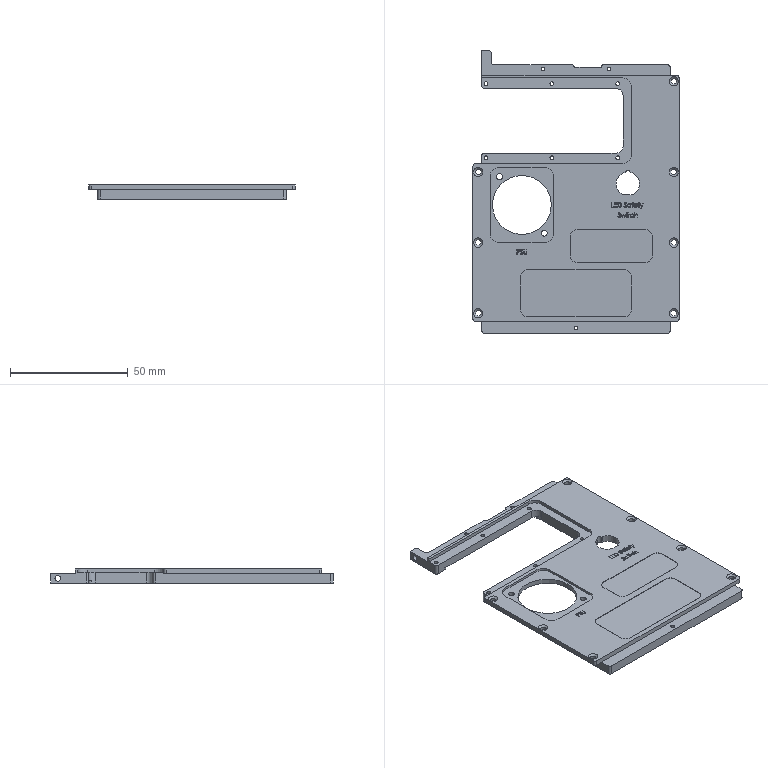NC program | NX | posted with a generic post | part box 87.5 x 120 x 6.001 mm
Lines 5364 to 6313 of 10039:
(ZLEVEL_PROFILE_STEEP , TOOL : D2-6-D4-50-3T-ROUGH)
N10684 T03 M6
N10686 G53
N10688 G17 G0 G90 X-21.7 Y-34.001 B0. C0. S6500 M3
N10690 G43 Z3. H3
N10692 Z-0.326
N10694 G94 G3 X-22.7 Y-35.001 R1. F1500.
N10696 G1 Y-36.95
N10698 X-20.751
N10700 G3 X-19.751 Y-35.95 R1.
N10702 G0 X-21.7 Y-34.001 Z-0.613
N10704 G3 X-22.7 Y-35.001 R1.
N10706 G1 Y-36.95
N10708 X-20.751
N10710 G3 X-19.751 Y-35.95 R1.
N10712 G0 X-21.7 Y-34.001 Z-0.9
N10714 G3 X-22.7 Y-35.001 R1.
N10716 G1 Y-36.95
N10718 X-20.751
N10720 G3 X-19.751 Y-35.95 R1.
N10722 G0 X-21.7 Y-34.001 Z-1.163
N10724 G3 X-22.7 Y-35.001 R1.
N10726 G1 Y-36.95
N10728 X-20.751
N10730 G3 X-19.751 Y-35.95 R1.
N10732 G0 X-21.7 Y-34.001 Z-1.489
N10734 G3 X-22.7 Y-35.001 R1.
N10736 G1 Y-36.95
N10738 X-20.751
N10740 G3 X-19.751 Y-35.95 R1.
N10742 G0 X-21.7 Y-34.001 Z-1.816
N10744 G3 X-22.7 Y-35.001 R1.
N10746 G1 Y-36.95
N10748 X-20.751
N10750 G3 X-19.751 Y-35.95 R1.
N10752 G0 X-21.7 Y-34.001 Z-2.087
N10754 G3 X-22.7 Y-35.001 R1.
N10756 G1 Y-36.95
N10758 X-20.751
N10760 G3 X-19.751 Y-35.95 R1.
N10762 G0 X-21.7 Y-34.001 Z-2.358
N10764 G3 X-22.7 Y-35.001 R1.
N10766 G1 Y-36.95
N10768 X-20.751
N10770 G3 X-19.751 Y-35.95 R1.
N10772 G0 X-21.7 Y-34.001 Z-2.629
N10774 G3 X-22.7 Y-35.001 R1.
N10776 G1 Y-36.95
N10778 X-20.751
N10780 G3 X-19.751 Y-35.95 R1.
N10782 G0 X-21.7 Y-34.001 Z-2.9
N10784 G3 X-22.7 Y-35.001 R1.
N10786 G1 Y-36.95
N10788 X-20.751
N10790 G3 X-19.751 Y-35.95 R1.
N10792 G0 Z3.1
N10794 X9.125
N10796 Z-0.326
N10798 G3 X10.125 Y-36.95 R1.
N10800 G1 X11.45
N10802 Y-36.75
N10804 G2 X11.574 Y-36.048 R2.05
N10806 G3 X11.126 Y-34.835 R1.
N10808 G0 X9.125 Y-35.95 Z-0.613
N10810 G3 X10.125 Y-36.95 R1.
N10812 G1 X11.45
N10814 Y-36.75
N10816 G2 X11.574 Y-36.048 R2.05
N10818 G3 X11.126 Y-34.835 R1.
N10820 G0 X9.125 Y-35.95 Z-0.9
N10822 G3 X10.125 Y-36.95 R1.
N10824 G1 X11.45
N10826 Y-36.75
N10828 G2 X11.574 Y-36.048 R2.05
N10830 G3 X11.126 Y-34.835 R1.
N10832 G0 X9.125 Y-35.95 Z-1.163
N10834 G3 X10.125 Y-36.95 R1.
N10836 G1 X11.45
N10838 Y-36.75
N10840 G2 X11.574 Y-36.048 R2.05
N10842 G3 X11.126 Y-34.835 R1.
N10844 G0 X9.125 Y-35.95 Z-1.489
N10846 G3 X10.125 Y-36.95 R1.
N10848 G1 X11.45
N10850 Y-36.75
N10852 G2 X11.574 Y-36.048 R2.05
N10854 G3 X11.126 Y-34.835 R1.
N10856 G0 X9.125 Y-35.95 Z-1.816
N10858 G3 X10.125 Y-36.95 R1.
N10860 G1 X11.45
N10862 Y-36.75
N10864 G2 X11.574 Y-36.048 R2.05
N10866 G3 X11.126 Y-34.835 R1.
N10868 G0 X9.125 Y-35.95 Z-2.087
N10870 G3 X10.125 Y-36.95 R1.
N10872 G1 X11.45
N10874 Y-36.75
N10876 G2 X11.574 Y-36.048 R2.05
N10878 G3 X11.126 Y-34.835 R1.
N10880 G0 X9.125 Y-35.95 Z-2.358
N10882 G3 X10.125 Y-36.95 R1.
N10884 G1 X11.45
N10886 Y-36.75
N10888 G2 X11.574 Y-36.048 R2.05
N10890 G3 X11.126 Y-34.835 R1.
N10892 G0 X9.125 Y-35.95 Z-2.629
N10894 G3 X10.125 Y-36.95 R1.
N10896 G1 X11.45
N10898 Y-36.75
N10900 G2 X11.574 Y-36.048 R2.05
N10902 G3 X11.126 Y-34.835 R1.
N10904 G0 X9.125 Y-35.95 Z-2.9
N10906 G3 X10.125 Y-36.95 R1.
N10908 G1 X11.45
N10910 Y-36.75
N10912 G2 X11.574 Y-36.048 R2.05
N10914 G3 X11.126 Y-34.835 R1.
N10916 G0 Z3.1
N10918 X11.435 Y-34.505
N10920 Z-0.326
N10922 G3 X12.675 Y-34.873 R1.
N10924 G2 X13.45 Y-34.701 R2.05
N10926 G1 Y-33.533
N10928 G3 X12.45 Y-32.533 R1.
N10930 G0 X11.435 Y-34.505 Z-0.613
N10932 G3 X12.675 Y-34.873 R1.
N10934 G2 X13.45 Y-34.701 R2.05
N10936 G1 Y-33.533
N10938 G3 X12.45 Y-32.533 R1.
N10940 G0 X11.435 Y-34.505 Z-0.9
N10942 G3 X12.675 Y-34.873 R1.
N10944 G2 X13.45 Y-34.701 R2.05
N10946 G1 Y-33.533
N10948 G3 X12.45 Y-32.533 R1.
N10950 G0 X11.435 Y-34.505 Z-1.163
N10952 G3 X12.675 Y-34.873 R1.
N10954 G2 X13.45 Y-34.701 R2.05
N10956 G1 Y-33.533
N10958 G3 X12.45 Y-32.533 R1.
N10960 G0 X11.435 Y-34.505 Z-1.489
N10962 G3 X12.675 Y-34.873 R1.
N10964 G2 X13.45 Y-34.701 R2.05
N10966 G1 Y-33.533
N10968 G3 X12.45 Y-32.533 R1.
N10970 G0 X11.435 Y-34.505 Z-1.816
N10972 G3 X12.675 Y-34.873 R1.
N10974 G2 X13.45 Y-34.701 R2.05
N10976 G1 Y-33.533
N10978 G3 X12.45 Y-32.533 R1.
N10980 G0 X11.435 Y-34.505 Z-2.087
N10982 G3 X12.675 Y-34.873 R1.
N10984 G2 X13.45 Y-34.701 R2.05
N10986 G1 Y-33.533
N10988 G3 X12.45 Y-32.533 R1.
N10990 G0 X11.435 Y-34.505 Z-2.358
N10992 G3 X12.675 Y-34.873 R1.
N10994 G2 X13.45 Y-34.701 R2.05
N10996 G1 Y-33.533
N10998 G3 X12.45 Y-32.533 R1.
N11000 G0 X11.435 Y-34.505 Z-2.629
N11002 G3 X12.675 Y-34.873 R1.
N11004 G2 X13.45 Y-34.701 R2.05
N11006 G1 Y-33.533
N11008 G3 X12.45 Y-32.533 R1.
N11010 G0 X11.435 Y-34.505 Z-2.9
N11012 G3 X12.675 Y-34.873 R1.
N11014 G2 X13.45 Y-34.701 R2.05
N11016 G1 Y-33.533
N11018 G3 X12.45 Y-32.533 R1.
N11020 G0 Z3.1
N11022 Y-15.967
N11024 Z-0.326
N11026 G3 X13.45 Y-14.967 R1.
N11028 G1 Y-13.799
N11030 G2 X12.675 Y-13.627 R2.05
N11032 G3 X11.435 Y-13.995 R1.
N11034 G0 X12.45 Y-15.967 Z-0.613
N11036 G3 X13.45 Y-14.967 R1.
N11038 G1 Y-13.799
N11040 G2 X12.675 Y-13.627 R2.05
N11042 G3 X11.435 Y-13.995 R1.
N11044 G0 X12.45 Y-15.967 Z-0.9
N11046 G3 X13.45 Y-14.967 R1.
N11048 G1 Y-13.799
N11050 G2 X12.675 Y-13.627 R2.05
N11052 G3 X11.435 Y-13.995 R1.
N11054 G0 X12.45 Y-15.967 Z-1.163
N11056 G3 X13.45 Y-14.967 R1.
N11058 G1 Y-13.799
N11060 G2 X12.675 Y-13.627 R2.05
N11062 G3 X11.435 Y-13.995 R1.
N11064 G0 X12.45 Y-15.967 Z-1.489
N11066 G3 X13.45 Y-14.967 R1.
N11068 G1 Y-13.799
N11070 G2 X12.675 Y-13.627 R2.05
N11072 G3 X11.435 Y-13.995 R1.
N11074 G0 X12.45 Y-15.967 Z-1.816
N11076 G3 X13.45 Y-14.967 R1.
N11078 G1 Y-13.799
N11080 G2 X12.675 Y-13.627 R2.05
N11082 G3 X11.435 Y-13.995 R1.
N11084 G0 X12.45 Y-15.967 Z-2.087
N11086 G3 X13.45 Y-14.967 R1.
N11088 G1 Y-13.799
N11090 G2 X12.675 Y-13.627 R2.05
N11092 G3 X11.435 Y-13.995 R1.
N11094 G0 X12.45 Y-15.967 Z-2.358
N11096 G3 X13.45 Y-14.967 R1.
N11098 G1 Y-13.799
N11100 G2 X12.675 Y-13.627 R2.05
N11102 G3 X11.435 Y-13.995 R1.
N11104 G0 X12.45 Y-15.967 Z-2.629
N11106 G3 X13.45 Y-14.967 R1.
N11108 G1 Y-13.799
N11110 G2 X12.675 Y-13.627 R2.05
N11112 G3 X11.435 Y-13.995 R1.
N11114 G0 X12.45 Y-15.967 Z-2.9
N11116 G3 X13.45 Y-14.967 R1.
N11118 G1 Y-13.799
N11120 G2 X12.675 Y-13.627 R2.05
N11122 G3 X11.435 Y-13.995 R1.
N11124 G0 Z3.1
N11126 X10.46 Y-11.999
N11128 Z-0.326
N11130 G3 X11.45 Y-10.999 R1.
N11132 G1 Y-9.05
N11134 X9.501
N11136 G3 X8.501 Y-10.05 R1.
N11138 G0 X10.46 Y-11.999 Z-0.613
N11140 G3 X11.45 Y-10.999 R1.
N11142 G1 Y-9.05
N11144 X9.501
N11146 G3 X8.501 Y-10.05 R1.
N11148 G0 X10.46 Y-11.999 Z-0.9
N11150 G3 X11.45 Y-10.999 R1.
N11152 G1 Y-9.05
N11154 X9.501
N11156 G3 X8.501 Y-10.05 R1.
N11158 G0 X10.46 Y-11.999 Z-1.163
N11160 G3 X11.45 Y-10.999 R1.
N11162 G1 Y-9.05
N11164 X9.501
N11166 G3 X8.501 Y-10.05 R1.
N11168 G0 X10.46 Y-11.999 Z-1.489
N11170 G3 X11.45 Y-10.999 R1.
N11172 G1 Y-9.05
N11174 X9.501
N11176 G3 X8.501 Y-10.05 R1.
N11178 G0 X10.46 Y-11.999 Z-1.816
N11180 G3 X11.45 Y-10.999 R1.
N11182 G1 Y-9.05
N11184 X9.501
N11186 G3 X8.501 Y-10.05 R1.
N11188 G0 X10.46 Y-11.999 Z-2.087
N11190 G3 X11.45 Y-10.999 R1.
N11192 G1 Y-9.05
N11194 X9.501
N11196 G3 X8.501 Y-10.05 R1.
N11198 G0 X10.46 Y-11.999 Z-2.358
N11200 G3 X11.45 Y-10.999 R1.
N11202 G1 Y-9.05
N11204 X9.501
N11206 G3 X8.501 Y-10.05 R1.
N11208 G0 X10.46 Y-11.999 Z-2.629
N11210 G3 X11.45 Y-10.999 R1.
N11212 G1 Y-9.05
N11214 X9.501
N11216 G3 X8.501 Y-10.05 R1.
N11218 G0 X10.46 Y-11.999 Z-2.9
N11220 G3 X11.45 Y-10.999 R1.
N11222 G1 Y-9.05
N11224 X9.501
N11226 G3 X8.501 Y-10.05 R1.
N11228 G0 Z3.1
N11230 X-19.751
N11232 Z-0.326
N11234 G3 X-20.751 Y-9.05 R1.
N11236 G1 X-22.7
N11238 Y-10.999
N11240 G3 X-21.7 Y-11.999 R1.
N11242 G0 X-19.751 Y-10.05 Z-0.613
N11244 G3 X-20.751 Y-9.05 R1.
N11246 G1 X-22.7
N11248 Y-10.999
N11250 G3 X-21.7 Y-11.999 R1.
N11252 G0 X-19.751 Y-10.05 Z-0.9
N11254 G3 X-20.751 Y-9.05 R1.
N11256 G1 X-22.7
N11258 Y-10.999
N11260 G3 X-21.7 Y-11.999 R1.
N11262 G0 X-19.751 Y-10.05 Z-1.163
N11264 G3 X-20.751 Y-9.05 R1.
N11266 G1 X-22.7
N11268 Y-10.999
N11270 G3 X-21.7 Y-11.999 R1.
N11272 G0 X-19.751 Y-10.05 Z-1.489
N11274 G3 X-20.751 Y-9.05 R1.
N11276 G1 X-22.7
N11278 Y-10.999
N11280 G3 X-21.7 Y-11.999 R1.
N11282 G0 X-19.751 Y-10.05 Z-1.816
N11284 G3 X-20.751 Y-9.05 R1.
N11286 G1 X-22.7
N11288 Y-10.999
N11290 G3 X-21.7 Y-11.999 R1.
N11292 G0 X-19.751 Y-10.05 Z-2.087
N11294 G3 X-20.751 Y-9.05 R1.
N11296 G1 X-22.7
N11298 Y-10.999
N11300 G3 X-21.7 Y-11.999 R1.
N11302 G0 X-19.751 Y-10.05 Z-2.358
N11304 G3 X-20.751 Y-9.05 R1.
N11306 G1 X-22.7
N11308 Y-10.999
N11310 G3 X-21.7 Y-11.999 R1.
N11312 G0 X-19.751 Y-10.05 Z-2.629
N11314 G3 X-20.751 Y-9.05 R1.
N11316 G1 X-22.7
N11318 Y-10.999
N11320 G3 X-21.7 Y-11.999 R1.
N11322 G0 X-19.751 Y-10.05 Z-2.9
N11324 G3 X-20.751 Y-9.05 R1.
N11326 G1 X-22.7
N11328 Y-10.999
N11330 G3 X-21.7 Y-11.999 R1.
N11332 G0 Z3.1
N11334 Y-2.001
N11336 Z-0.326
N11338 G3 X-22.7 Y-3.001 R1.
N11340 G1 Y-4.95
N11342 X-20.751
N11344 G3 X-19.751 Y-3.95 R1.
N11346 G0 X-21.7 Y-2.001 Z-0.613
N11348 G3 X-22.7 Y-3.001 R1.
N11350 G1 Y-4.95
N11352 X-20.751
N11354 G3 X-19.751 Y-3.95 R1.
N11356 G0 X-21.7 Y-2.001 Z-0.9
N11358 G3 X-22.7 Y-3.001 R1.
N11360 G1 Y-4.95
N11362 X-20.751
N11364 G3 X-19.751 Y-3.95 R1.
N11366 G0 X-21.7 Y-2.001 Z-1.163
N11368 G3 X-22.7 Y-3.001 R1.
N11370 G1 Y-4.95
N11372 X-20.751
N11374 G3 X-19.751 Y-3.95 R1.
N11376 G0 X-21.7 Y-2.001 Z-1.489
N11378 G3 X-22.7 Y-3.001 R1.
N11380 G1 Y-4.95
N11382 X-20.751
N11384 G3 X-19.751 Y-3.95 R1.
N11386 G0 X-21.7 Y-2.001 Z-1.816
N11388 G3 X-22.7 Y-3.001 R1.
N11390 G1 Y-4.95
N11392 X-20.751
N11394 G3 X-19.751 Y-3.95 R1.
N11396 G0 X-21.7 Y-2.001 Z-2.087
N11398 G3 X-22.7 Y-3.001 R1.
N11400 G1 Y-4.95
N11402 X-20.751
N11404 G3 X-19.751 Y-3.95 R1.
N11406 G0 X-21.7 Y-2.001 Z-2.358
N11408 G3 X-22.7 Y-3.001 R1.
N11410 G1 Y-4.95
N11412 X-20.751
N11414 G3 X-19.751 Y-3.95 R1.
N11416 G0 X-21.7 Y-2.001 Z-2.629
N11418 G3 X-22.7 Y-3.001 R1.
N11420 G1 Y-4.95
N11422 X-20.751
N11424 G3 X-19.751 Y-3.95 R1.
N11426 G0 X-21.7 Y-2.001 Z-2.9
N11428 G3 X-22.7 Y-3.001 R1.
N11430 G1 Y-4.95
N11432 X-20.751
N11434 G3 X-19.751 Y-3.95 R1.
N11436 G0 Z3.1
N11438 X10.501
N11440 Z-0.326
N11442 G3 X11.501 Y-4.95 R1.
N11444 G1 X13.45
N11446 Y-3.001
N11448 G3 X12.45 Y-2.001 R1.
N11450 G0 X10.501 Y-3.95 Z-0.613
N11452 G3 X11.501 Y-4.95 R1.
N11454 G1 X13.45
N11456 Y-3.001
N11458 G3 X12.45 Y-2.001 R1.
N11460 G0 X10.501 Y-3.95 Z-0.9
N11462 G3 X11.501 Y-4.95 R1.
N11464 G1 X13.45
N11466 Y-3.001
N11468 G3 X12.45 Y-2.001 R1.
N11470 G0 X10.501 Y-3.95 Z-1.163
N11472 G3 X11.501 Y-4.95 R1.
N11474 G1 X13.45
N11476 Y-3.001
N11478 G3 X12.45 Y-2.001 R1.
N11480 G0 X10.501 Y-3.95 Z-1.489
N11482 G3 X11.501 Y-4.95 R1.
N11484 G1 X13.45
N11486 Y-3.001
N11488 G3 X12.45 Y-2.001 R1.
N11490 G0 X10.501 Y-3.95 Z-1.816
N11492 G3 X11.501 Y-4.95 R1.
N11494 G1 X13.45
N11496 Y-3.001
N11498 G3 X12.45 Y-2.001 R1.
N11500 G0 X10.501 Y-3.95 Z-2.087
N11502 G3 X11.501 Y-4.95 R1.
N11504 G1 X13.45
N11506 Y-3.001
N11508 G3 X12.45 Y-2.001 R1.
N11510 G0 X10.501 Y-3.95 Z-2.358
N11512 G3 X11.501 Y-4.95 R1.
N11514 G1 X13.45
N11516 Y-3.001
N11518 G3 X12.45 Y-2.001 R1.
N11520 G0 X10.501 Y-3.95 Z-2.629
N11522 G3 X11.501 Y-4.95 R1.
N11524 G1 X13.45
N11526 Y-3.001
N11528 G3 X12.45 Y-2.001 R1.
N11530 G0 X10.501 Y-3.95 Z-2.9
N11532 G3 X11.501 Y-4.95 R1.
N11534 G1 X13.45
N11536 Y-3.001
N11538 G3 X12.45 Y-2.001 R1.
N11540 G0 Z3.1
N11542 Y2.501
N11544 Z-0.326
N11546 G3 X13.45 Y3.501 R1.
N11548 G1 Y5.45
N11550 X11.501
N11552 G3 X10.501 Y4.45 R1.
N11554 G0 X12.45 Y2.501 Z-0.613
N11556 G3 X13.45 Y3.501 R1.
N11558 G1 Y5.45
N11560 X11.501
N11562 G3 X10.501 Y4.45 R1.
N11564 G0 X12.45 Y2.501 Z-0.9
N11566 G3 X13.45 Y3.501 R1.
N11568 G1 Y5.45
N11570 X11.501
N11572 G3 X10.501 Y4.45 R1.
N11574 G0 X12.45 Y2.501 Z-1.163
N11576 G3 X13.45 Y3.501 R1.
N11578 G1 Y5.45
N11580 X11.501
N11582 G3 X10.501 Y4.45 R1.
N11584 G0 X12.45 Y2.501 Z-1.489
N11586 G3 X13.45 Y3.501 R1.
N11588 G1 Y5.45
N11590 X11.501
N11592 G3 X10.501 Y4.45 R1.
N11594 G0 X12.45 Y2.501 Z-1.816
N11596 G3 X13.45 Y3.501 R1.
N11598 G1 Y5.45
N11600 X11.501
N11602 G3 X10.501 Y4.45 R1.
N11604 G0 X12.45 Y2.501 Z-2.087
N11606 G3 X13.45 Y3.501 R1.
N11608 G1 Y5.45
N11610 X11.501
N11612 G3 X10.501 Y4.45 R1.
N11614 G0 X12.45 Y2.501 Z-2.358
N11616 G3 X13.45 Y3.501 R1.
N11618 G1 Y5.45
N11620 X11.501
N11622 G3 X10.501 Y4.45 R1.
N11624 G0 X12.45 Y2.501 Z-2.629
N11626 G3 X13.45 Y3.501 R1.
N11628 G1 Y5.45
N11630 X11.501
N11632 G3 X10.501 Y4.45 R1.
N11634 G0 X12.45 Y2.501 Z-2.9
N11636 G3 X13.45 Y3.501 R1.
N11638 G1 Y5.45
N11640 X11.501
N11642 G3 X10.501 Y4.45 R1.
N11644 G0 Z3.1
N11646 X-19.751
N11648 Z-0.326
N11650 G3 X-20.751 Y5.45 R1.
N11652 G1 X-22.7
N11654 Y3.501
N11656 G3 X-21.7 Y2.501 R1.
N11658 G0 X-19.751 Y4.45 Z-0.613
N11660 G3 X-20.751 Y5.45 R1.
N11662 G1 X-22.7
N11664 Y3.501
N11666 G3 X-21.7 Y2.501 R1.
N11668 G0 X-19.751 Y4.45 Z-0.9
N11670 G3 X-20.751 Y5.45 R1.
N11672 G1 X-22.7
N11674 Y3.501
N11676 G3 X-21.7 Y2.501 R1.
N11678 G0 X-19.751 Y4.45 Z-1.163
N11680 G3 X-20.751 Y5.45 R1.
N11682 G1 X-22.7
N11684 Y3.501
N11686 G3 X-21.7 Y2.501 R1.
N11688 G0 X-19.751 Y4.45 Z-1.489
N11690 G3 X-20.751 Y5.45 R1.
N11692 G1 X-22.7
N11694 Y3.501
N11696 G3 X-21.7 Y2.501 R1.
N11698 G0 X-19.751 Y4.45 Z-1.816
N11700 G3 X-20.751 Y5.45 R1.
N11702 G1 X-22.7
N11704 Y3.501
N11706 G3 X-21.7 Y2.501 R1.
N11708 G0 X-19.751 Y4.45 Z-2.087
N11710 G3 X-20.751 Y5.45 R1.
N11712 G1 X-22.7
N11714 Y3.501
N11716 G3 X-21.7 Y2.501 R1.
N11718 G0 X-19.751 Y4.45 Z-2.358
N11720 G3 X-20.751 Y5.45 R1.
N11722 G1 X-22.7
N11724 Y3.501
N11726 G3 X-21.7 Y2.501 R1.
N11728 G0 X-19.751 Y4.45 Z-2.629
N11730 G3 X-20.751 Y5.45 R1.
N11732 G1 X-22.7
N11734 Y3.501
N11736 G3 X-21.7 Y2.501 R1.
N11738 G0 X-19.751 Y4.45 Z-2.9
N11740 G3 X-20.751 Y5.45 R1.
N11742 G1 X-22.7
N11744 Y3.501
N11746 G3 X-21.7 Y2.501 R1.
N11748 G0 Z3.1
N11750 Y12.499
N11752 Z-0.326
N11754 G3 X-22.7 Y11.499 R1.
N11756 G1 Y9.55
N11758 X-20.751
N11760 G3 X-19.751 Y10.55 R1.
N11762 G0 X-21.7 Y12.499 Z-0.613
N11764 G3 X-22.7 Y11.499 R1.
N11766 G1 Y9.55
N11768 X-20.751
N11770 G3 X-19.751 Y10.55 R1.
N11772 G0 X-21.7 Y12.499 Z-0.9
N11774 G3 X-22.7 Y11.499 R1.
N11776 G1 Y9.55
N11778 X-20.751
N11780 G3 X-19.751 Y10.55 R1.
N11782 G0 X-21.7 Y12.499 Z-1.163
N11784 G3 X-22.7 Y11.499 R1.
N11786 G1 Y9.55
N11788 X-20.751
N11790 G3 X-19.751 Y10.55 R1.
N11792 G0 X-21.7 Y12.499 Z-1.489
N11794 G3 X-22.7 Y11.499 R1.
N11796 G1 Y9.55
N11798 X-20.751
N11800 G3 X-19.751 Y10.55 R1.
N11802 G0 X-21.7 Y12.499 Z-1.816
N11804 G3 X-22.7 Y11.499 R1.
N11806 G1 Y9.55
N11808 X-20.751
N11810 G3 X-19.751 Y10.55 R1.
N11812 G0 X-21.7 Y12.499 Z-2.087
N11814 G3 X-22.7 Y11.499 R1.
N11816 G1 Y9.55
N11818 X-20.751
N11820 G3 X-19.751 Y10.55 R1.
N11822 G0 X-21.7 Y12.499 Z-2.358
N11824 G3 X-22.7 Y11.499 R1.
N11826 G1 Y9.55
N11828 X-20.751
N11830 G3 X-19.751 Y10.55 R1.
N11832 G0 X-21.7 Y12.499 Z-2.629
N11834 G3 X-22.7 Y11.499 R1.
N11836 G1 Y9.55
N11838 X-20.751
N11840 G3 X-19.751 Y10.55 R1.
N11842 G0 X-21.7 Y12.499 Z-2.9
N11844 G3 X-22.7 Y11.499 R1.
N11846 G1 Y9.55
N11848 X-20.751
N11850 G3 X-19.751 Y10.55 R1.
N11852 G0 Z3.1
N11854 X10.501
N11856 Z-0.326
N11858 G3 X11.501 Y9.55 R1.
N11860 G1 X13.45
N11862 Y11.499
N11864 G3 X12.45 Y12.499 R1.
N11866 G0 X10.501 Y10.55 Z-0.613
N11868 G3 X11.501 Y9.55 R1.
N11870 G1 X13.45
N11872 Y11.499
N11874 G3 X12.45 Y12.499 R1.
N11876 G0 X10.501 Y10.55 Z-0.9
N11878 G3 X11.501 Y9.55 R1.
N11880 G1 X13.45
N11882 Y11.499
N11884 G3 X12.45 Y12.499 R1.
N11886 G0 X10.501 Y10.55 Z-1.163
N11888 G3 X11.501 Y9.55 R1.
N11890 G1 X13.45
N11892 Y11.499
N11894 G3 X12.45 Y12.499 R1.
N11896 G0 X10.501 Y10.55 Z-1.489
N11898 G3 X11.501 Y9.55 R1.
N11900 G1 X13.45
N11902 Y11.499
N11904 G3 X12.45 Y12.499 R1.
N11906 G0 X10.501 Y10.55 Z-1.816
N11908 G3 X11.501 Y9.55 R1.
N11910 G1 X13.45
N11912 Y11.499
N11914 G3 X12.45 Y12.499 R1.
N11916 G0 X10.501 Y10.55 Z-2.087
N11918 G3 X11.501 Y9.55 R1.
N11920 G1 X13.45
N11922 Y11.499
N11924 G3 X12.45 Y12.499 R1.
N11926 G0 X10.501 Y10.55 Z-2.358
N11928 G3 X11.501 Y9.55 R1.
N11930 G1 X13.45
N11932 Y11.499
N11934 G3 X12.45 Y12.499 R1.
N11936 G0 X10.501 Y10.55 Z-2.629
N11938 G3 X11.501 Y9.55 R1.
N11940 G1 X13.45
N11942 Y11.499
N11944 G3 X12.45 Y12.499 R1.
N11946 G0 X10.501 Y10.55 Z-2.9
N11948 G3 X11.501 Y9.55 R1.
N11950 G1 X13.45
N11952 Y11.499
N11954 G3 X12.45 Y12.499 R1.
N11956 G0 Z3.1
N11958 Y12.033
N11960 Z-0.326
N11962 G3 X13.45 Y13.033 R1.
N11964 G1 Y14.201
N11966 G2 X12.675 Y14.373 R2.05
N11968 G3 X11.435 Y14.005 R1.
N11970 G0 X12.45 Y12.033 Z-0.613
N11972 G3 X13.45 Y13.033 R1.
N11974 G1 Y14.201
N11976 G2 X12.675 Y14.373 R2.05
N11978 G3 X11.435 Y14.005 R1.
N11980 G0 X12.45 Y12.033 Z-0.9
N11982 G3 X13.45 Y13.033 R1.
N11984 G1 Y14.201
N11986 G2 X12.675 Y14.373 R2.05
N11988 G3 X11.435 Y14.005 R1.
N11990 G0 X12.45 Y12.033 Z-1.163
N11992 G3 X13.45 Y13.033 R1.
N11994 G1 Y14.201
N11996 G2 X12.675 Y14.373 R2.05
N11998 G3 X11.435 Y14.005 R1.
N12000 G0 X12.45 Y12.033 Z-1.489
N12002 G3 X13.45 Y13.033 R1.
N12004 G1 Y14.201
N12006 G2 X12.675 Y14.373 R2.05
N12008 G3 X11.435 Y14.005 R1.
N12010 G0 X12.45 Y12.033 Z-1.816
N12012 G3 X13.45 Y13.033 R1.
N12014 G1 Y14.201
N12016 G2 X12.675 Y14.373 R2.05
N12018 G3 X11.435 Y14.005 R1.
N12020 G0 X12.45 Y12.033 Z-2.087
N12022 G3 X13.45 Y13.033 R1.
N12024 G1 Y14.201
N12026 G2 X12.675 Y14.373 R2.05
N12028 G3 X11.435 Y14.005 R1.
N12030 G0 X12.45 Y12.033 Z-2.358
N12032 G3 X13.45 Y13.033 R1.
N12034 G1 Y14.201
N12036 G2 X12.675 Y14.373 R2.05
N12038 G3 X11.435 Y14.005 R1.
N12040 G0 X12.45 Y12.033 Z-2.629
N12042 G3 X13.45 Y13.033 R1.
N12044 G1 Y14.201
N12046 G2 X12.675 Y14.373 R2.05
N12048 G3 X11.435 Y14.005 R1.
N12050 G0 X12.45 Y12.033 Z-2.9
N12052 G3 X13.45 Y13.033 R1.
N12054 G1 Y14.201
N12056 G2 X12.675 Y14.373 R2.05
N12058 G3 X11.435 Y14.005 R1.
N12060 G0 Z3.1
N12062 Y21.495
N12064 Z-0.326
N12066 G3 X12.675 Y21.127 R1.
N12068 G2 X13.45 Y21.299 R2.05
N12070 G1 Y22.467
N12072 G3 X12.45 Y23.467 R1.
N12074 G0 X11.435 Y21.495 Z-0.613
N12076 G3 X12.675 Y21.127 R1.
N12078 G2 X13.45 Y21.299 R2.05
N12080 G1 Y22.467
N12082 G3 X12.45 Y23.467 R1.
N12084 G0 X11.435 Y21.495 Z-0.9
N12086 G3 X12.675 Y21.127 R1.
N12088 G2 X13.45 Y21.299 R2.05
N12090 G1 Y22.467
N12092 G3 X12.45 Y23.467 R1.
N12094 G0 X11.435 Y21.495 Z-1.163
N12096 G3 X12.675 Y21.127 R1.
N12098 G2 X13.45 Y21.299 R2.05
N12100 G1 Y22.467
N12102 G3 X12.45 Y23.467 R1.
N12104 G0 X11.435 Y21.495 Z-1.489
N12106 G3 X12.675 Y21.127 R1.
N12108 G2 X13.45 Y21.299 R2.05
N12110 G1 Y22.467
N12112 G3 X12.45 Y23.467 R1.
N12114 G0 X11.435 Y21.495 Z-1.816
N12116 G3 X12.675 Y21.127 R1.
N12118 G2 X13.45 Y21.299 R2.05
N12120 G1 Y22.467
N12122 G3 X12.45 Y23.467 R1.
N12124 G0 X11.435 Y21.495 Z-2.087
N12126 G3 X12.675 Y21.127 R1.
N12128 G2 X13.45 Y21.299 R2.05
N12130 G1 Y22.467
N12132 G3 X12.45 Y23.467 R1.
N12134 G0 X11.435 Y21.495 Z-2.358
N12136 G3 X12.675 Y21.127 R1.
N12138 G2 X13.45 Y21.299 R2.05
N12140 G1 Y22.467
N12142 G3 X12.45 Y23.467 R1.
N12144 G0 X11.435 Y21.495 Z-2.629
N12146 G3 X12.675 Y21.127 R1.
N12148 G2 X13.45 Y21.299 R2.05
N12150 G1 Y22.467
N12152 G3 X12.45 Y23.467 R1.
N12154 G0 X11.435 Y21.495 Z-2.9
N12156 G3 X12.675 Y21.127 R1.
N12158 G2 X13.45 Y21.299 R2.05
N12160 G1 Y22.467
N12162 G3 X12.45 Y23.467 R1.
N12164 G0 Z3.1
N12166 Y34.001
N12168 Z-0.326
N12170 G3 X13.45 Y35.001 R1.
N12172 G1 Y36.95
N12174 X11.501
N12176 G3 X10.501 Y35.95 R1.
N12178 G0 X12.45 Y34.001 Z-0.613
N12180 G3 X13.45 Y35.001 R1.
N12182 G1 Y36.95
N12184 X11.501
N12186 G3 X10.501 Y35.95 R1.
N12188 G0 X12.45 Y34.001 Z-0.9
N12190 G3 X13.45 Y35.001 R1.
N12192 G1 Y36.95
N12194 X11.501
N12196 G3 X10.501 Y35.95 R1.
N12198 G0 X12.45 Y34.001 Z-1.163
N12200 G3 X13.45 Y35.001 R1.
N12202 G1 Y36.95
N12204 X11.501
N12206 G3 X10.501 Y35.95 R1.
N12208 G0 X12.45 Y34.001 Z-1.489
N12210 G3 X13.45 Y35.001 R1.
N12212 G1 Y36.95
N12214 X11.501
N12216 G3 X10.501 Y35.95 R1.
N12218 G0 X12.45 Y34.001 Z-1.816
N12220 G3 X13.45 Y35.001 R1.
N12222 G1 Y36.95
N12224 X11.501
N12226 G3 X10.501 Y35.95 R1.
N12228 G0 X12.45 Y34.001 Z-2.087
N12230 G3 X13.45 Y35.001 R1.
N12232 G1 Y36.95
N12234 X11.501
N12236 G3 X10.501 Y35.95 R1.
N12238 G0 X12.45 Y34.001 Z-2.358
N12240 G3 X13.45 Y35.001 R1.
N12242 G1 Y36.95
N12244 X11.501
N12246 G3 X10.501 Y35.95 R1.
N12248 G0 X12.45 Y34.001 Z-2.629
N12250 G3 X13.45 Y35.001 R1.
N12252 G1 Y36.95
N12254 X11.501
N12256 G3 X10.501 Y35.95 R1.
N12258 G0 X12.45 Y34.001 Z-2.9
N12260 G3 X13.45 Y35.001 R1.
N12262 G1 Y36.95
N12264 X11.501
N12266 G3 X10.501 Y35.95 R1.
N12268 G0 Z3.1
N12270 X-19.751
N12272 Z-0.326
N12274 G3 X-20.751 Y36.95 R1.
N12276 G1 X-22.7
N12278 Y35.001
N12280 G3 X-21.7 Y34.001 R1.
N12282 G0 X-19.751 Y35.95 Z-0.613
N12284 G3 X-20.751 Y36.95 R1.
N12286 G1 X-22.7
N12288 Y35.001
N12290 G3 X-21.7 Y34.001 R1.
N12292 G0 X-19.751 Y35.95 Z-0.9
N12294 G3 X-20.751 Y36.95 R1.
N12296 G1 X-22.7
N12298 Y35.001
N12300 G3 X-21.7 Y34.001 R1.
N12302 G0 X-19.751 Y35.95 Z-1.163
N12304 G3 X-20.751 Y36.95 R1.
N12306 G1 X-22.7
N12308 Y35.001
N12310 G3 X-21.7 Y34.001 R1.
N12312 G0 X-19.751 Y35.95 Z-1.489
N12314 G3 X-20.751 Y36.95 R1.
N12316 G1 X-22.7
N12318 Y35.001
N12320 G3 X-21.7 Y34.001 R1.
N12322 G0 X-19.751 Y35.95 Z-1.816
N12324 G3 X-20.751 Y36.95 R1.
N12326 G1 X-22.7
N12328 Y35.001
N12330 G3 X-21.7 Y34.001 R1.
N12332 G0 X-19.751 Y35.95 Z-2.087
N12334 G3 X-20.751 Y36.95 R1.
N12336 G1 X-22.7
N12338 Y35.001
N12340 G3 X-21.7 Y34.001 R1.
N12342 G0 X-19.751 Y35.95 Z-2.358
N12344 G3 X-20.751 Y36.95 R1.
N12346 G1 X-22.7
N12348 Y35.001
N12350 G3 X-21.7 Y34.001 R1.
N12352 G0 X-19.751 Y35.95 Z-2.629
N12354 G3 X-20.751 Y36.95 R1.
N12356 G1 X-22.7
N12358 Y35.001
N12360 G3 X-21.7 Y34.001 R1.
N12362 G0 X-19.751 Y35.95 Z-2.9
N12364 G3 X-20.751 Y36.95 R1.
N12366 G1 X-22.7
N12368 Y35.001
N12370 G3 X-21.7 Y34.001 R1.
N12372 G0 Z3.1
N12374 X-52.238 Y4.45
N12376 Z-0.326
N12378 G3 X-53.238 Y5.45 R1.
N12380 G1 X-56.95
N12382 Y3.549
N12384 G2 X-55.206 Y2.492 R2.05
N12386 G3 X-53.997 Y2.033 R1.
N12388 G0 X-52.238 Y4.45 Z-0.613
N12390 G3 X-53.238 Y5.45 R1.
N12392 G1 X-56.95
N12394 Y3.549
N12396 G2 X-55.206 Y2.492 R2.05
N12398 G3 X-53.997 Y2.033 R1.
N12400 G0 X-52.238 Y4.45 Z-0.9
N12402 G3 X-53.238 Y5.45 R1.
N12404 G1 X-56.95
N12406 Y3.549
N12408 G2 X-55.206 Y2.492 R2.05
N12410 G3 X-53.997 Y2.033 R1.
N12412 G0 X-52.238 Y4.45 Z-1.163
N12414 G3 X-53.238 Y5.45 R1.
N12416 G1 X-56.95
N12418 Y3.549
N12420 G2 X-55.206 Y2.492 R2.05
N12422 G3 X-53.997 Y2.033 R1.
N12424 G0 X-52.238 Y4.45 Z-1.489
N12426 G3 X-53.238 Y5.45 R1.
N12428 G1 X-56.95
N12430 Y3.549
N12432 G2 X-55.206 Y2.492 R2.05
N12434 G3 X-53.997 Y2.033 R1.
N12436 G0 X-52.238 Y4.45 Z-1.816
N12438 G3 X-53.238 Y5.45 R1.
N12440 G1 X-56.95
N12442 Y3.549
N12444 G2 X-55.206 Y2.492 R2.05
N12446 G3 X-53.997 Y2.033 R1.
N12448 G0 X-52.238 Y4.45 Z-2.087
N12450 G3 X-53.238 Y5.45 R1.
N12452 G1 X-56.95
N12454 Y3.549
N12456 G2 X-55.206 Y2.492 R2.05
N12458 G3 X-53.997 Y2.033 R1.
N12460 G0 X-52.238 Y4.45 Z-2.358
N12462 G3 X-53.238 Y5.45 R1.
N12464 G1 X-56.95
N12466 Y3.549
N12468 G2 X-55.206 Y2.492 R2.05
N12470 G3 X-53.997 Y2.033 R1.
N12472 G0 X-52.238 Y4.45 Z-2.629
N12474 G3 X-53.238 Y5.45 R1.
N12476 G1 X-56.95
N12478 Y3.549
N12480 G2 X-55.206 Y2.492 R2.05
N12482 G3 X-53.997 Y2.033 R1.
N12484 G0 X-52.238 Y4.45 Z-2.9
N12486 G3 X-53.238 Y5.45 R1.
N12488 G1 X-56.95
N12490 Y3.549
N12492 G2 X-55.206 Y2.492 R2.05
N12494 G3 X-53.997 Y2.033 R1.
N12496 G0 Z3.1
N12498 X-54.935 Y-3.745
N12500 Z-0.326
N12502 G3 X-56.175 Y-3.377 R1.
N12504 G2 X-56.95 Y-3.549 R2.05
N12506 G1 Y-4.717
N12508 G3 X-55.95 Y-5.717 R1.
N12510 G0 X-54.935 Y-3.745 Z-0.613
N12512 G3 X-56.175 Y-3.377 R1.
N12514 G2 X-56.95 Y-3.549 R2.05
N12516 G1 Y-4.717
N12518 G3 X-55.95 Y-5.717 R1.
N12520 G0 X-54.935 Y-3.745 Z-0.9
N12522 G3 X-56.175 Y-3.377 R1.
N12524 G2 X-56.95 Y-3.549 R2.05
N12526 G1 Y-4.717
N12528 G3 X-55.95 Y-5.717 R1.
N12530 G0 X-54.935 Y-3.745 Z-1.163
N12532 G3 X-56.175 Y-3.377 R1.
N12534 G2 X-56.95 Y-3.549 R2.05
N12536 G1 Y-4.717
N12538 G3 X-55.95 Y-5.717 R1.
N12540 G0 X-54.935 Y-3.745 Z-1.489
N12542 G3 X-56.175 Y-3.377 R1.
N12544 G2 X-56.95 Y-3.549 R2.05
N12546 G1 Y-4.717
N12548 G3 X-55.95 Y-5.717 R1.
N12550 G0 X-54.935 Y-3.745 Z-1.816
N12552 G3 X-56.175 Y-3.377 R1.
N12554 G2 X-56.95 Y-3.549 R2.05
N12556 G1 Y-4.717
N12558 G3 X-55.95 Y-5.717 R1.
N12560 G0 X-54.935 Y-3.745 Z-2.087
N12562 G3 X-56.175 Y-3.377 R1.
N12564 G2 X-56.95 Y-3.549 R2.05
N12566 G1 Y-4.717
N12568 G3 X-55.95 Y-5.717 R1.
N12570 G0 X-54.935 Y-3.745 Z-2.358
N12572 G3 X-56.175 Y-3.377 R1.
N12574 G2 X-56.95 Y-3.549 R2.05
N12576 G1 Y-4.717